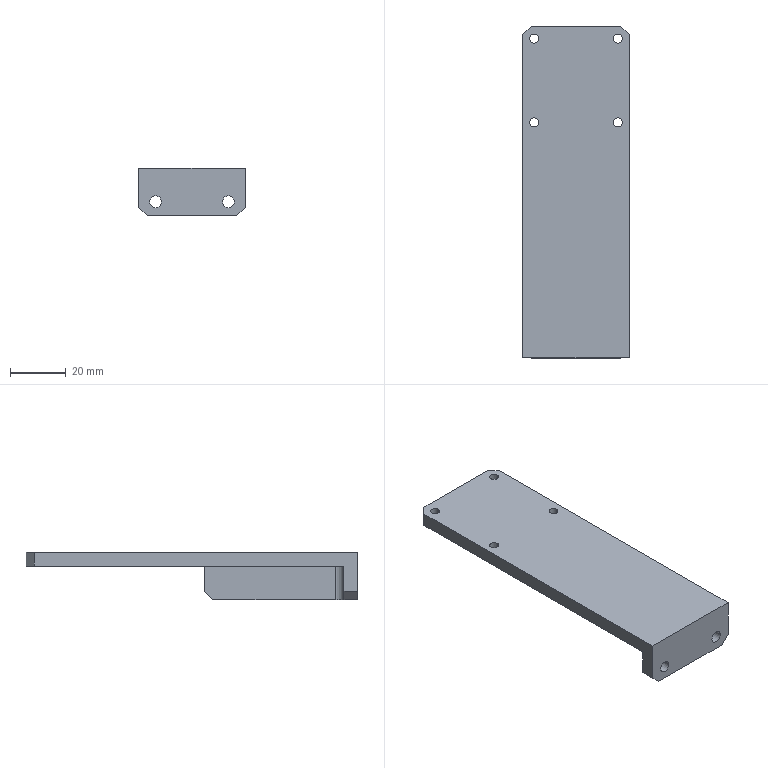NC program | NX | posted with a generic post | part box 38.1 x 118.8 x 17 mm
Lines 1 to 1973 of 2704, first 1714 of 1959 lines:
N10 G17 G21 G94 G90
(FLOOR_WALL_COPY_COPY , TOOL : D80)
N12 T19 M6
N14 G54
N16 G17 G0 G90 X-104.4 Y0. S6500 M3
N18 G43 Z30. H19
N20 Z5.
N22 G94 G1 Z2. F1500.
N24 X-99.4
N26 X99.4
N28 X104.4
N30 Z5.
N32 G0 Z30.
N34 X-104.4
N36 Z4.
N38 G1 Z1.
N40 X-99.4
N42 X99.4
N44 X104.4
N46 Z4.
N48 G0 Z30.
N50 X-104.4
N52 Z3.
N54 G1 Z0.
N56 X-99.4
N58 X99.4
N60 X104.4
N62 Z3.
N64 G0 Z30.
N66 M5
(FLOOR_WALL , TOOL : D10)
N68 T15 M6
N70 G54
N72 G17 G0 G90 X63.9 Y-22.864 S9500 M3
N74 G43 Z30. H15
N76 Z-8.9
N78 G94 G1 Z-10.9 F1000.
N80 Y-22.788 Z-11.283
N82 Y-22.571 Z-11.607
N84 Y-22.246 Z-11.824
N86 Y-21.864 Z-11.9
N88 Y-18.621
N90 Y18.518 F3000.
N92 X63.909 Y18.625
N94 X63.827 Y18.694
N96 X63.572 Y18.949
N98 G3 X63.402 Y18.878 R0.1
N100 G1 Y-19.016
N102 X63.41 Y-19.123
N104 X63.328 Y-19.193
N106 X63.074 Y-19.447
N108 G2 X62.903 Y-19.377 R0.1
N110 G1 Y19.515
N112 X62.912 Y19.622
N114 X62.83 Y19.691
N116 X62.575 Y19.946
N118 G3 X62.405 Y19.875 R0.1
N120 G1 Y-20.013
N122 X62.413 Y-20.12
N124 X62.332 Y-20.189
N126 X62.077 Y-20.444
N128 G2 X61.906 Y-20.374 R0.1
N130 G1 Y20.512
N132 X61.915 Y20.619
N134 X61.833 Y20.688
N136 X61.578 Y20.943
N138 G3 X61.408 Y20.872 R0.1
N140 G1 Y-21.01
N142 X61.416 Y-21.117
N144 X61.335 Y-21.186
N146 X61.08 Y-21.441
N148 G2 X60.909 Y-21.371 R0.1
N150 G1 Y21.509
N152 X60.918 Y21.615
N154 X60.836 Y21.685
N156 X60.581 Y21.94
N158 G3 X60.411 Y21.869 R0.1
N160 G1 Y-22.007
N162 X60.419 Y-22.114
N164 X60.338 Y-22.183
N166 X60.083 Y-22.438
N168 G2 X59.912 Y-22.367 R0.1
N170 G1 Y22.505
N172 X59.921 Y22.612
N174 X59.839 Y22.682
N176 X59.584 Y22.937
N178 G3 X59.414 Y22.866 R0.1
N180 G1 Y-23.004
N182 X59.423 Y-23.111
N184 X59.341 Y-23.18
N186 X59.086 Y-23.435
N188 G2 X58.915 Y-23.364 R0.1
N190 G1 Y23.502
N192 X58.924 Y23.609
N194 X58.842 Y23.679
N196 X58.588 Y23.934
N198 G3 X58.417 Y23.863 R0.1
N200 G1 Y-23.826
N202 G2 X58.193 Y-24.05 R0.224
N204 G1 X58.168
N206 G2 X57.918 Y-23.8 R0.25
N208 G1 Y23.826
N210 G3 X57.694 Y24.05 R0.224
N212 G1 X57.67
N214 G3 X57.42 Y23.8 R0.25
N216 G1 Y-23.826
N218 G2 X57.196 Y-24.05 R0.224
N220 G1 X57.172
N222 G2 X56.922 Y-23.8 R0.25
N224 G1 Y23.826
N226 G3 X56.697 Y24.05 R0.224
N228 G1 X56.673
N230 G3 X56.423 Y23.8 R0.25
N232 G1 Y-23.826
N234 G2 X56.199 Y-24.05 R0.224
N236 G1 X56.175
N238 G2 X55.925 Y-23.8 R0.25
N240 G1 Y23.826
N242 G3 X55.7 Y24.05 R0.224
N244 G1 X55.676
N246 G3 X55.426 Y23.8 R0.25
N248 G1 Y-23.826
N250 G2 X55.202 Y-24.05 R0.224
N252 G1 X55.178
N254 G2 X54.928 Y-23.8 R0.25
N256 G1 Y23.826
N258 G3 X54.703 Y24.05 R0.224
N260 G1 X54.679
N262 G3 X54.429 Y23.8 R0.25
N264 G1 Y-23.826
N266 G2 X54.205 Y-24.05 R0.224
N268 G1 X54.181
N270 G2 X53.931 Y-23.8 R0.25
N272 G1 Y23.826
N274 G3 X53.707 Y24.05 R0.224
N276 G1 X53.682
N278 G3 X53.432 Y23.8 R0.25
N280 G1 Y-23.826
N282 G2 X53.208 Y-24.05 R0.224
N284 G1 X53.184
N286 G2 X52.934 Y-23.8 R0.25
N288 G1 Y23.826
N290 G3 X52.71 Y24.05 R0.224
N292 G1 X52.685
N294 G3 X52.435 Y23.8 R0.25
N296 G1 Y-23.826
N298 G2 X52.211 Y-24.05 R0.224
N300 G1 X52.187
N302 G2 X51.937 Y-23.8 R0.25
N304 G1 Y23.826
N306 G3 X51.713 Y24.05 R0.224
N308 G1 X51.689
N310 G3 X51.439 Y23.8 R0.25
N312 G1 Y-23.826
N314 G2 X51.214 Y-24.05 R0.224
N316 G1 X51.19
N318 G2 X50.94 Y-23.8 R0.25
N320 G1 Y23.826
N322 G3 X50.716 Y24.05 R0.224
N324 G1 X50.692
N326 G3 X50.442 Y23.8 R0.25
N328 G1 Y-23.826
N330 G2 X50.217 Y-24.05 R0.224
N332 G1 X50.193
N334 G2 X49.943 Y-23.8 R0.25
N336 G1 Y23.826
N338 G3 X49.719 Y24.05 R0.224
N340 G1 X49.695
N342 G3 X49.445 Y23.8 R0.25
N344 G1 Y-23.826
N346 G2 X49.22 Y-24.05 R0.224
N348 G1 X49.196
N350 G2 X48.946 Y-23.8 R0.25
N352 G1 Y23.826
N354 G3 X48.722 Y24.05 R0.224
N356 G1 X48.698
N358 G3 X48.448 Y23.8 R0.25
N360 G1 Y-23.826
N362 G2 X48.223 Y-24.05 R0.224
N364 G1 X48.199
N366 G2 X47.949 Y-23.8 R0.25
N368 G1 Y23.826
N370 G3 X47.725 Y24.05 R0.224
N372 G1 X47.701
N374 G3 X47.451 Y23.8 R0.25
N376 G1 Y-23.826
N378 G2 X47.227 Y-24.05 R0.224
N380 G1 X47.202
N382 G2 X46.952 Y-23.8 R0.25
N384 G1 Y23.826
N386 G3 X46.728 Y24.05 R0.224
N388 G1 X46.704
N390 G3 X46.454 Y23.8 R0.25
N392 G1 Y-23.826
N394 G2 X46.23 Y-24.05 R0.224
N396 G1 X46.205
N398 G2 X45.955 Y-23.8 R0.25
N400 G1 Y23.826
N402 G3 X45.731 Y24.05 R0.224
N404 G1 X45.707
N406 G3 X45.457 Y23.8 R0.25
N408 G1 Y-23.826
N410 G2 X45.233 Y-24.05 R0.224
N412 G1 X45.209
N414 G2 X44.959 Y-23.8 R0.25
N416 G1 Y23.826
N418 G3 X44.734 Y24.05 R0.224
N420 G1 X44.71
N422 G3 X44.46 Y23.8 R0.25
N424 G1 Y-23.826
N426 G2 X44.236 Y-24.05 R0.224
N428 G1 X44.212
N430 G2 X43.962 Y-23.8 R0.25
N432 G1 Y23.826
N434 G3 X43.737 Y24.05 R0.224
N436 G1 X43.713
N438 G3 X43.463 Y23.8 R0.25
N440 G1 Y-23.826
N442 G2 X43.239 Y-24.05 R0.224
N444 G1 X43.215
N446 G2 X42.965 Y-23.8 R0.25
N448 G1 Y23.826
N450 G3 X42.74 Y24.05 R0.224
N452 G1 X42.716
N454 G3 X42.466 Y23.8 R0.25
N456 G1 Y-23.826
N458 G2 X42.242 Y-24.05 R0.224
N460 G1 X42.218
N462 G2 X41.968 Y-23.8 R0.25
N464 G1 Y23.826
N466 G3 X41.744 Y24.05 R0.224
N468 G1 X41.719
N470 G3 X41.469 Y23.8 R0.25
N472 G1 Y-23.826
N474 G2 X41.245 Y-24.05 R0.224
N476 G1 X41.221
N478 G2 X40.971 Y-23.8 R0.25
N480 G1 Y23.826
N482 G3 X40.747 Y24.05 R0.224
N484 G1 X40.722
N486 G3 X40.472 Y23.8 R0.25
N488 G1 Y-23.826
N490 G2 X40.248 Y-24.05 R0.224
N492 G1 X40.224
N494 G2 X39.974 Y-23.8 R0.25
N496 G1 Y23.826
N498 G3 X39.75 Y24.05 R0.224
N500 G1 X39.726
N502 G3 X39.476 Y23.8 R0.25
N504 G1 Y-23.826
N506 G2 X39.251 Y-24.05 R0.224
N508 G1 X39.227
N510 G2 X38.977 Y-23.8 R0.25
N512 G1 Y23.826
N514 G3 X38.753 Y24.05 R0.224
N516 G1 X38.729
N518 G3 X38.479 Y23.8 R0.25
N520 G1 Y-23.826
N522 G2 X38.254 Y-24.05 R0.224
N524 G1 X38.23
N526 G2 X37.98 Y-23.8 R0.25
N528 G1 Y23.826
N530 G3 X37.756 Y24.05 R0.224
N532 G1 X37.732
N534 G3 X37.482 Y23.8 R0.25
N536 G1 Y-23.826
N538 G2 X37.257 Y-24.05 R0.224
N540 G1 X37.233
N542 G2 X36.983 Y-23.8 R0.25
N544 G1 Y23.826
N546 G3 X36.759 Y24.05 R0.224
N548 G1 X36.735
N550 G3 X36.485 Y23.8 R0.25
N552 G1 Y-23.826
N554 G2 X36.26 Y-24.05 R0.224
N556 G1 X36.236
N558 G2 X35.986 Y-23.8 R0.25
N560 G1 Y23.826
N562 G3 X35.762 Y24.05 R0.224
N564 G1 X35.738
N566 G3 X35.488 Y23.8 R0.25
N568 G1 Y-23.826
N570 G2 X35.264 Y-24.05 R0.224
N572 G1 X35.239
N574 G2 X34.989 Y-23.8 R0.25
N576 G1 Y23.826
N578 G3 X34.765 Y24.05 R0.224
N580 G1 X34.741
N582 G3 X34.491 Y23.8 R0.25
N584 G1 Y-23.826
N586 G2 X34.267 Y-24.05 R0.224
N588 G1 X34.243
N590 G2 X33.993 Y-23.8 R0.25
N592 G1 Y23.826
N594 G3 X33.768 Y24.05 R0.224
N596 G1 X33.744
N598 G3 X33.494 Y23.8 R0.25
N600 G1 Y-23.826
N602 G2 X33.27 Y-24.05 R0.224
N604 G1 X33.246
N606 G2 X32.996 Y-23.8 R0.25
N608 G1 Y23.826
N610 G3 X32.771 Y24.05 R0.224
N612 G1 X32.747
N614 G3 X32.497 Y23.8 R0.25
N616 G1 Y-23.826
N618 G2 X32.273 Y-24.05 R0.224
N620 G1 X32.249
N622 G2 X31.999 Y-23.8 R0.25
N624 G1 Y23.826
N626 G3 X31.774 Y24.05 R0.224
N628 G1 X31.75
N630 G3 X31.5 Y23.8 R0.25
N632 G1 Y-23.826
N634 G2 X31.276 Y-24.05 R0.224
N636 G1 X31.252
N638 G2 X31.002 Y-23.8 R0.25
N640 G1 Y23.826
N642 G3 X30.777 Y24.05 R0.224
N644 G1 X30.753
N646 G3 X30.503 Y23.8 R0.25
N648 G1 Y-23.826
N650 G2 X30.279 Y-24.05 R0.224
N652 G1 X30.255
N654 G2 X30.005 Y-23.8 R0.25
N656 G1 Y23.826
N658 G3 X29.781 Y24.05 R0.224
N660 G1 X29.756
N662 G3 X29.506 Y23.8 R0.25
N664 G1 Y-23.826
N666 G2 X29.282 Y-24.05 R0.224
N668 G1 X29.258
N670 G2 X29.008 Y-23.8 R0.25
N672 G1 Y23.826
N674 G3 X28.784 Y24.05 R0.224
N676 G1 X28.759
N678 G3 X28.509 Y23.8 R0.25
N680 G1 Y-23.826
N682 G2 X28.285 Y-24.05 R0.224
N684 G1 X28.261
N686 G2 X28.011 Y-23.8 R0.25
N688 G1 Y23.826
N690 G3 X27.787 Y24.05 R0.224
N692 G1 X27.763
N694 G3 X27.513 Y23.8 R0.25
N696 G1 Y-23.826
N698 G2 X27.288 Y-24.05 R0.224
N700 G1 X27.264
N702 G2 X27.014 Y-23.8 R0.25
N704 G1 Y23.826
N706 G3 X26.79 Y24.05 R0.224
N708 G1 X26.766
N710 G3 X26.516 Y23.8 R0.25
N712 G1 Y-23.826
N714 G2 X26.291 Y-24.05 R0.224
N716 G1 X26.267
N718 G2 X26.017 Y-23.8 R0.25
N720 G1 Y23.826
N722 G3 X25.793 Y24.05 R0.224
N724 G1 X25.769
N726 G3 X25.519 Y23.8 R0.25
N728 G1 Y-23.826
N730 G2 X25.294 Y-24.05 R0.224
N732 G1 X25.27
N734 G2 X25.02 Y-23.8 R0.25
N736 G1 Y23.826
N738 G3 X24.796 Y24.05 R0.224
N740 G1 X24.772
N742 G3 X24.522 Y23.8 R0.25
N744 G1 Y-23.826
N746 G2 X24.297 Y-24.05 R0.224
N748 G1 X24.273
N750 G2 X24.023 Y-23.8 R0.25
N752 G1 Y23.826
N754 G3 X23.799 Y24.05 R0.224
N756 G1 X23.775
N758 G3 X23.525 Y23.8 R0.25
N760 G1 Y-23.826
N762 G2 X23.301 Y-24.05 R0.224
N764 G1 X23.276
N766 G2 X23.026 Y-23.8 R0.25
N768 G1 Y23.826
N770 G3 X22.802 Y24.05 R0.224
N772 G1 X22.778
N774 G3 X22.528 Y23.8 R0.25
N776 G1 Y-23.826
N778 G2 X22.304 Y-24.05 R0.224
N780 G1 X22.28
N782 G2 X22.03 Y-23.8 R0.25
N784 G1 Y23.826
N786 G3 X21.805 Y24.05 R0.224
N788 G1 X21.781
N790 G3 X21.531 Y23.8 R0.25
N792 G1 Y-23.826
N794 G2 X21.307 Y-24.05 R0.224
N796 G1 X21.283
N798 G2 X21.033 Y-23.8 R0.25
N800 G1 Y23.826
N802 G3 X20.808 Y24.05 R0.224
N804 G1 X20.784
N806 G3 X20.534 Y23.8 R0.25
N808 G1 Y-23.826
N810 G2 X20.31 Y-24.05 R0.224
N812 G1 X20.286
N814 G2 X20.036 Y-23.8 R0.25
N816 G1 Y23.826
N818 G3 X19.811 Y24.05 R0.224
N820 G1 X19.787
N822 G3 X19.537 Y23.8 R0.25
N824 G1 Y-23.826
N826 G2 X19.313 Y-24.05 R0.224
N828 G1 X19.289
N830 G2 X19.039 Y-23.8 R0.25
N832 G1 Y23.826
N834 G3 X18.814 Y24.05 R0.224
N836 G1 X18.79
N838 G3 X18.54 Y23.8 R0.25
N840 G1 Y-23.826
N842 G2 X18.316 Y-24.05 R0.224
N844 G1 X18.292
N846 G2 X18.042 Y-23.8 R0.25
N848 G1 Y23.826
N850 G3 X17.818 Y24.05 R0.224
N852 G1 X17.793
N854 G3 X17.543 Y23.8 R0.25
N856 G1 Y-23.826
N858 G2 X17.319 Y-24.05 R0.224
N860 G1 X17.295
N862 G2 X17.045 Y-23.8 R0.25
N864 G1 Y23.826
N866 G3 X16.821 Y24.05 R0.224
N868 G1 X16.796
N870 G3 X16.546 Y23.8 R0.25
N872 G1 Y-23.826
N874 G2 X16.322 Y-24.05 R0.224
N876 G1 X16.298
N878 G2 X16.048 Y-23.8 R0.25
N880 G1 Y23.826
N882 G3 X15.824 Y24.05 R0.224
N884 G1 X15.8
N886 G3 X15.55 Y23.8 R0.25
N888 G1 Y-23.826
N890 G2 X15.325 Y-24.05 R0.224
N892 G1 X15.301
N894 G2 X15.051 Y-23.8 R0.25
N896 G1 Y23.826
N898 G3 X14.827 Y24.05 R0.224
N900 G1 X14.803
N902 G3 X14.553 Y23.8 R0.25
N904 G1 Y-23.826
N906 G2 X14.328 Y-24.05 R0.224
N908 G1 X14.304
N910 G2 X14.054 Y-23.8 R0.25
N912 G1 Y23.826
N914 G3 X13.83 Y24.05 R0.224
N916 G1 X13.806
N918 G3 X13.556 Y23.8 R0.25
N920 G1 Y-23.826
N922 G2 X13.331 Y-24.05 R0.224
N924 G1 X13.307
N926 G2 X13.057 Y-23.8 R0.25
N928 G1 Y23.826
N930 G3 X12.833 Y24.05 R0.224
N932 G1 X12.809
N934 G3 X12.559 Y23.8 R0.25
N936 G1 Y-23.826
N938 G2 X12.335 Y-24.05 R0.224
N940 G1 X12.31
N942 G2 X12.06 Y-23.8 R0.25
N944 G1 Y23.826
N946 G3 X11.836 Y24.05 R0.224
N948 G1 X11.812
N950 G3 X11.562 Y23.8 R0.25
N952 G1 Y-23.826
N954 G2 X11.338 Y-24.05 R0.224
N956 G1 X11.313
N958 G2 X11.063 Y-23.8 R0.25
N960 G1 Y23.826
N962 G3 X10.839 Y24.05 R0.224
N964 G1 X10.815
N966 G3 X10.565 Y23.8 R0.25
N968 G1 Y-23.826
N970 G2 X10.341 Y-24.05 R0.224
N972 G1 X10.317
N974 G2 X10.067 Y-23.8 R0.25
N976 G1 Y23.826
N978 G3 X9.842 Y24.05 R0.224
N980 G1 X9.818
N982 G3 X9.568 Y23.8 R0.25
N984 G1 Y-23.826
N986 G2 X9.344 Y-24.05 R0.224
N988 G1 X9.32
N990 G2 X9.07 Y-23.8 R0.25
N992 G1 Y23.826
N994 G3 X8.845 Y24.05 R0.224
N996 G1 X8.821
N998 G3 X8.571 Y23.8 R0.25
N1000 G1 Y-23.826
N1002 G2 X8.347 Y-24.05 R0.224
N1004 G1 X8.323
N1006 G2 X8.073 Y-23.8 R0.25
N1008 G1 Y23.826
N1010 G3 X7.848 Y24.05 R0.224
N1012 G1 X7.824
N1014 G3 X7.574 Y23.8 R0.25
N1016 G1 Y-23.826
N1018 G2 X7.35 Y-24.05 R0.224
N1020 G1 X7.326
N1022 G2 X7.076 Y-23.8 R0.25
N1024 G1 Y23.826
N1026 G3 X6.851 Y24.05 R0.224
N1028 G1 X6.827
N1030 G3 X6.577 Y23.8 R0.25
N1032 G1 Y-23.826
N1034 G2 X6.353 Y-24.05 R0.224
N1036 G1 X6.329
N1038 G2 X6.079 Y-23.8 R0.25
N1040 G1 Y23.826
N1042 G3 X5.855 Y24.05 R0.224
N1044 G1 X5.83
N1046 G3 X5.58 Y23.8 R0.25
N1048 G1 Y-23.826
N1050 G2 X5.356 Y-24.05 R0.224
N1052 G1 X5.332
N1054 G2 X5.082 Y-23.8 R0.25
N1056 G1 Y23.826
N1058 G3 X4.858 Y24.05 R0.224
N1060 G1 X4.833
N1062 G3 X4.583 Y23.8 R0.25
N1064 G1 Y-23.826
N1066 G2 X4.359 Y-24.05 R0.224
N1068 G1 X4.335
N1070 G2 X4.085 Y-23.8 R0.25
N1072 G1 Y23.826
N1074 G3 X3.861 Y24.05 R0.224
N1076 G1 X3.837
N1078 G3 X3.587 Y23.8 R0.25
N1080 G1 Y-23.826
N1082 G2 X3.362 Y-24.05 R0.224
N1084 G1 X3.338
N1086 G2 X3.088 Y-23.8 R0.25
N1088 G1 Y23.826
N1090 G3 X2.864 Y24.05 R0.224
N1092 G1 X2.84
N1094 G3 X2.59 Y23.8 R0.25
N1096 G1 Y-23.826
N1098 G2 X2.365 Y-24.05 R0.224
N1100 G1 X2.341
N1102 G2 X2.091 Y-23.8 R0.25
N1104 G1 Y23.826
N1106 G3 X1.867 Y24.05 R0.224
N1108 G1 X1.843
N1110 G3 X1.593 Y23.8 R0.25
N1112 G1 Y-23.826
N1114 G2 X1.368 Y-24.05 R0.224
N1116 G1 X1.344
N1118 G2 X1.094 Y-23.8 R0.25
N1120 G1 Y23.826
N1122 G3 X0.87 Y24.05 R0.224
N1124 G1 X0.846
N1126 G3 X0.596 Y23.8 R0.25
N1128 G1 Y9.374
N1130 G2 X0.372 Y9.15 R0.224
N1132 G1 X0.347
N1134 G2 X0.097 Y9.4 R0.25
N1136 G1 Y23.826
N1138 G3 X-0.127 Y24.05 R0.224
N1140 G1 X-0.151
N1142 G3 X-0.401 Y23.8 R0.25
N1144 G1 Y9.399
N1146 G2 X-0.65 Y9.15 R0.249
N1148 G1 X-0.675
N1150 G2 X-0.9 Y9.374 R0.224
N1152 G1 Y23.826
N1154 G3 X-1.124 Y24.05 R0.224
N1156 G1 X-1.148
N1158 G3 X-1.398 Y23.8 R0.25
N1160 G1 Y9.399
N1162 G2 X-1.647 Y9.15 R0.249
N1164 G1 X-1.672
N1166 G2 X-1.896 Y9.374 R0.224
N1168 G1 Y23.826
N1170 G3 X-2.121 Y24.05 R0.224
N1172 G1 X-2.145
N1174 G3 X-2.395 Y23.8 R0.25
N1176 G1 Y9.399
N1178 G2 X-2.644 Y9.15 R0.249
N1180 G1 X-2.669
N1182 G2 X-2.893 Y9.374 R0.224
N1184 G1 Y23.826
N1186 G3 X-3.118 Y24.05 R0.224
N1188 G1 X-3.142
N1190 G3 X-3.392 Y23.8 R0.25
N1192 G1 Y9.374
N1194 G2 X-3.616 Y9.15 R0.224
N1196 G1 X-3.64
N1198 G2 X-3.89 Y9.4 R0.25
N1200 G1 Y23.826
N1202 G3 X-4.115 Y24.05 R0.224
N1204 G1 X-4.139
N1206 G3 X-4.389 Y23.8 R0.25
N1208 G1 Y9.374
N1210 G2 X-4.613 Y9.15 R0.224
N1212 G1 X-4.637
N1214 G2 X-4.887 Y9.4 R0.25
N1216 G1 Y23.826
N1218 G3 X-5.112 Y24.05 R0.224
N1220 G1 X-5.136
N1222 G3 X-5.386 Y23.8 R0.25
N1224 G1 Y9.374
N1226 G2 X-5.61 Y9.15 R0.224
N1228 G1 X-5.634
N1230 G2 X-5.884 Y9.4 R0.25
N1232 G1 Y23.826
N1234 G3 X-6.108 Y24.05 R0.224
N1236 G1 X-6.133
N1238 G3 X-6.383 Y23.8 R0.25
N1240 G1 Y9.374
N1242 G2 X-6.607 Y9.15 R0.224
N1244 G1 X-6.631
N1246 G2 X-6.881 Y9.4 R0.25
N1248 G1 Y23.826
N1250 G3 X-7.105 Y24.05 R0.224
N1252 G1 X-7.13
N1254 G3 X-7.38 Y23.8 R0.25
N1256 G1 Y9.374
N1258 G2 X-7.604 Y9.15 R0.224
N1260 G1 X-7.628
N1262 G2 X-7.878 Y9.4 R0.25
N1264 G1 Y23.826
N1266 G3 X-8.102 Y24.05 R0.224
N1268 G1 X-8.126
N1270 G3 X-8.376 Y23.8 R0.25
N1272 G1 Y9.374
N1274 G2 X-8.601 Y9.15 R0.224
N1276 G1 X-8.625
N1278 G2 X-8.875 Y9.4 R0.25
N1280 G1 Y23.826
N1282 G3 X-9.099 Y24.05 R0.224
N1284 G1 X-9.123
N1286 G3 X-9.373 Y23.8 R0.25
N1288 G1 Y9.374
N1290 G2 X-9.598 Y9.15 R0.224
N1292 G1 X-9.622
N1294 G2 X-9.872 Y9.4 R0.25
N1296 G1 Y23.826
N1298 G3 X-10.096 Y24.05 R0.224
N1300 G1 X-10.12
N1302 G3 X-10.37 Y23.8 R0.25
N1304 G1 Y9.374
N1306 G2 X-10.595 Y9.15 R0.224
N1308 G1 X-10.619
N1310 G2 X-10.869 Y9.4 R0.25
N1312 G1 Y23.826
N1314 G3 X-11.093 Y24.05 R0.224
N1316 G1 X-11.117
N1318 G3 X-11.367 Y23.8 R0.25
N1320 G1 Y9.374
N1322 G2 X-11.591 Y9.15 R0.224
N1324 G1 X-11.616
N1326 G2 X-11.866 Y9.4 R0.25
N1328 G1 Y23.826
N1330 G3 X-12.09 Y24.05 R0.224
N1332 G1 X-12.114
N1334 G3 X-12.364 Y23.8 R0.25
N1336 G1 Y9.374
N1338 G2 X-12.588 Y9.15 R0.224
N1340 G1 X-12.613
N1342 G2 X-12.863 Y9.4 R0.25
N1344 G1 Y23.826
N1346 G3 X-13.087 Y24.05 R0.224
N1348 G1 X-13.111
N1350 G3 X-13.361 Y23.8 R0.25
N1352 G1 Y9.399
N1354 G2 X-13.61 Y9.15 R0.249
N1356 G1 X-13.635
N1358 G2 X-13.859 Y9.374 R0.224
N1360 G1 Y23.826
N1362 G3 X-14.084 Y24.05 R0.224
N1364 G1 X-14.108
N1366 G3 X-14.358 Y23.8 R0.25
N1368 G1 Y9.374
N1370 G2 X-14.582 Y9.15 R0.224
N1372 G1 X-14.606
N1374 G2 X-14.856 Y9.4 R0.25
N1376 G1 Y23.826
N1378 G3 X-15.081 Y24.05 R0.224
N1380 G1 X-15.105
N1382 G3 X-15.355 Y23.8 R0.25
N1384 G1 Y9.374
N1386 G2 X-15.579 Y9.15 R0.224
N1388 G1 X-15.603
N1390 G2 X-15.853 Y9.4 R0.25
N1392 G1 Y23.826
N1394 G3 X-16.078 Y24.05 R0.224
N1396 G1 X-16.102
N1398 G3 X-16.352 Y23.8 R0.25
N1400 G1 Y9.374
N1402 G2 X-16.576 Y9.15 R0.224
N1404 G1 X-16.6
N1406 G2 X-16.85 Y9.4 R0.25
N1408 G1 Y23.826
N1410 G3 X-17.075 Y24.05 R0.224
N1412 G1 X-17.099
N1414 G3 X-17.349 Y23.8 R0.25
N1416 G1 Y9.374
N1418 G2 X-17.573 Y9.15 R0.224
N1420 G1 X-17.597
N1422 G2 X-17.847 Y9.4 R0.25
N1424 G1 Y23.826
N1426 G3 X-18.071 Y24.05 R0.224
N1428 G1 X-18.096
N1430 G3 X-18.346 Y23.8 R0.25
N1432 G1 Y9.374
N1434 G2 X-18.57 Y9.15 R0.224
N1436 G1 X-18.594
N1438 G2 X-18.844 Y9.4 R0.25
N1440 G1 Y23.826
N1442 G3 X-19.068 Y24.05 R0.224
N1444 G1 X-19.093
N1446 G3 X-19.343 Y23.8 R0.25
N1448 G1 Y9.374
N1450 G2 X-19.567 Y9.15 R0.224
N1452 G1 X-19.591
N1454 G2 X-19.841 Y9.4 R0.25
N1456 G1 Y23.826
N1458 G3 X-20.065 Y24.05 R0.224
N1460 G1 X-20.089
N1462 G3 X-20.339 Y23.8 R0.25
N1464 G1 Y9.374
N1466 G2 X-20.564 Y9.15 R0.224
N1468 G1 X-20.588
N1470 G2 X-20.838 Y9.4 R0.25
N1472 G1 Y23.826
N1474 G3 X-21.062 Y24.05 R0.224
N1476 G1 X-21.086
N1478 G3 X-21.336 Y23.8 R0.25
N1480 G1 Y9.374
N1482 G2 X-21.561 Y9.15 R0.224
N1484 G1 X-21.585
N1486 G2 X-21.835 Y9.4 R0.25
N1488 G1 Y23.826
N1490 G3 X-22.059 Y24.05 R0.224
N1492 G1 X-22.083
N1494 G3 X-22.333 Y23.8 R0.25
N1496 G1 Y9.374
N1498 G2 X-22.558 Y9.15 R0.224
N1500 G1 X-22.582
N1502 G2 X-22.832 Y9.4 R0.25
N1504 G1 Y23.826
N1506 G3 X-23.056 Y24.05 R0.224
N1508 G1 X-23.08
N1510 G3 X-23.33 Y23.8 R0.25
N1512 G1 Y9.399
N1514 G2 X-23.579 Y9.15 R0.249
N1516 G1 X-23.604
N1518 G2 X-23.829 Y9.374 R0.224
N1520 G1 Y23.826
N1522 G3 X-24.053 Y24.05 R0.224
N1524 G1 X-24.077
N1526 G3 X-24.327 Y23.8 R0.25
N1528 G1 Y9.374
N1530 G2 X-24.551 Y9.15 R0.224
N1532 G1 X-24.576
N1534 G2 X-24.826 Y9.4 R0.25
N1536 G1 Y23.826
N1538 G3 X-25.05 Y24.05 R0.224
N1540 G1 X-25.074
N1542 G3 X-25.324 Y23.8 R0.25
N1544 G1 Y9.374
N1546 G2 X-25.548 Y9.15 R0.224
N1548 G1 X-25.572
N1550 G2 X-25.822 Y9.4 R0.25
N1552 G1 Y23.826
N1554 G3 X-26.047 Y24.05 R0.224
N1556 G1 X-26.071
N1558 G3 X-26.321 Y23.8 R0.25
N1560 G1 Y9.374
N1562 G2 X-26.545 Y9.15 R0.224
N1564 G1 X-26.569
N1566 G2 X-26.819 Y9.4 R0.25
N1568 G1 Y23.826
N1570 G3 X-27.044 Y24.05 R0.224
N1572 G1 X-27.068
N1574 G3 X-27.318 Y23.8 R0.25
N1576 G1 Y9.374
N1578 G2 X-27.542 Y9.15 R0.224
N1580 G1 X-27.566
N1582 G2 X-27.816 Y9.4 R0.25
N1584 G1 Y23.826
N1586 G3 X-28.041 Y24.05 R0.224
N1588 G1 X-28.065
N1590 G3 X-28.315 Y23.8 R0.25
N1592 G1 Y9.374
N1594 G2 X-28.539 Y9.15 R0.224
N1596 G1 X-28.563
N1598 G2 X-28.813 Y9.4 R0.25
N1600 G1 Y23.826
N1602 G3 X-29.038 Y24.05 R0.224
N1604 G1 X-29.062
N1606 G3 X-29.312 Y23.8 R0.25
N1608 G1 Y9.399
N1610 G2 X-29.561 Y9.15 R0.249
N1612 G1 X-29.586
N1614 G2 X-29.81 Y9.374 R0.224
N1616 G1 Y23.826
N1618 G3 X-30.034 Y24.05 R0.224
N1620 G1 X-30.059
N1622 G3 X-30.309 Y23.8 R0.25
N1624 G1 Y9.374
N1626 G2 X-30.533 Y9.15 R0.224
N1628 G1 X-30.557
N1630 G2 X-30.807 Y9.4 R0.25
N1632 G1 Y23.826
N1634 G3 X-31.031 Y24.05 R0.224
N1636 G1 X-31.055
N1638 G3 X-31.305 Y23.8 R0.25
N1640 G1 Y9.374
N1642 G2 X-31.53 Y9.15 R0.224
N1644 G1 X-31.554
N1646 G2 X-31.804 Y9.4 R0.25
N1648 G1 Y23.826
N1650 G3 X-32.028 Y24.05 R0.224
N1652 G1 X-32.052
N1654 G3 X-32.302 Y23.8 R0.25
N1656 G1 Y9.374
N1658 G2 X-32.527 Y9.15 R0.224
N1660 G1 X-32.551
N1662 G2 X-32.801 Y9.4 R0.25
N1664 G1 Y23.826
N1666 G3 X-33.025 Y24.05 R0.224
N1668 G1 X-33.049
N1670 G3 X-33.299 Y23.8 R0.25
N1672 G1 Y9.374
N1674 G2 X-33.524 Y9.15 R0.224
N1676 G1 X-33.548
N1678 G2 X-33.798 Y9.4 R0.25
N1680 G1 Y23.826
N1682 G3 X-34.022 Y24.05 R0.224
N1684 G1 X-34.046
N1686 G3 X-34.296 Y23.8 R0.25
N1688 G1 Y9.374
N1690 G2 X-34.521 Y9.15 R0.224
N1692 G1 X-34.545
N1694 G2 X-34.795 Y9.4 R0.25
N1696 G1 Y23.826
N1698 G3 X-35.019 Y24.05 R0.224
N1700 G1 X-35.043
N1702 G3 X-35.293 Y23.8 R0.25
N1704 G1 Y9.374
N1706 G2 X-35.517 Y9.15 R0.224
N1708 G1 X-35.542
N1710 G2 X-35.792 Y9.4 R0.25
N1712 G1 Y23.826
N1714 G3 X-36.016 Y24.05 R0.224
N1716 G1 X-36.04
N1718 G3 X-36.29 Y23.8 R0.25
N1720 G1 Y9.374
N1722 G2 X-36.514 Y9.15 R0.224
N1724 G1 X-36.539
N1726 G2 X-36.789 Y9.4 R0.25
N1728 G1 Y23.826
N1730 G3 X-37.013 Y24.05 R0.224
N1732 G1 X-37.037
N1734 G3 X-37.287 Y23.8 R0.25
N1736 G1 Y9.374
N1738 G2 X-37.511 Y9.15 R0.224
N1740 G1 X-37.535
N1742 G2 X-37.785 Y9.4 R0.25
N1744 G1 Y23.826
N1746 G3 X-38.01 Y24.05 R0.224
N1748 G1 X-38.034
N1750 G3 X-38.284 Y23.8 R0.25
N1752 G1 Y9.374
N1754 G2 X-38.508 Y9.15 R0.224
N1756 G1 X-38.532
N1758 G2 X-38.782 Y9.4 R0.25
N1760 G1 Y23.826
N1762 G3 X-39.007 Y24.05 R0.224
N1764 G1 X-39.031
N1766 G3 X-39.281 Y23.8 R0.25
N1768 G1 Y9.374
N1770 G2 X-39.505 Y9.15 R0.224
N1772 G1 X-39.529
N1774 G2 X-39.779 Y9.4 R0.25
N1776 G1 Y23.826
N1778 G3 X-40.004 Y24.05 R0.224
N1780 G1 X-40.028
N1782 G3 X-40.278 Y23.8 R0.25
N1784 G1 Y9.374
N1786 G2 X-40.502 Y9.15 R0.224
N1788 G1 X-40.526
N1790 G2 X-40.776 Y9.4 R0.25
N1792 G1 Y23.826
N1794 G3 X-41.001 Y24.05 R0.224
N1796 G1 X-41.025
N1798 G3 X-41.275 Y23.8 R0.25
N1800 G1 Y9.374
N1802 G2 X-41.499 Y9.15 R0.224
N1804 G1 X-41.523
N1806 G2 X-41.773 Y9.4 R0.25
N1808 G1 Y23.826
N1810 G3 X-41.997 Y24.05 R0.224
N1812 G1 X-42.022
N1814 G3 X-42.272 Y23.8 R0.25
N1816 G1 Y9.374
N1818 G2 X-42.496 Y9.15 R0.224
N1820 G1 X-42.52
N1822 G2 X-42.77 Y9.4 R0.25
N1824 G1 Y23.826
N1826 G3 X-42.994 Y24.05 R0.224
N1828 G1 X-43.018
N1830 G3 X-43.268 Y23.8 R0.25
N1832 G1 Y9.374
N1834 G2 X-43.493 Y9.15 R0.224
N1836 G1 X-43.517
N1838 G2 X-43.767 Y9.4 R0.25
N1840 G1 Y23.826
N1842 G3 X-43.991 Y24.05 R0.224
N1844 G1 X-44.015
N1846 G3 X-44.265 Y23.8 R0.25
N1848 G1 Y9.374
N1850 G2 X-44.49 Y9.15 R0.224
N1852 G1 X-44.514
N1854 G2 X-44.764 Y9.4 R0.25
N1856 G1 Y23.826
N1858 G3 X-44.988 Y24.05 R0.224
N1860 G1 X-45.012
N1862 G3 X-45.262 Y23.8 R0.25
N1864 G1 Y9.374
N1866 G2 X-45.487 Y9.15 R0.224
N1868 G1 X-45.511
N1870 G2 X-45.761 Y9.4 R0.25
N1872 G1 Y23.826
N1874 G3 X-45.985 Y24.05 R0.224
N1876 G1 X-46.009
N1878 G3 X-46.259 Y23.8 R0.25
N1880 G1 Y9.374
N1882 G2 X-46.484 Y9.15 R0.224
N1884 G1 X-46.508
N1886 G2 X-46.758 Y9.4 R0.25
N1888 G1 Y23.826
N1890 G3 X-46.982 Y24.05 R0.224
N1892 G1 X-47.006
N1894 G3 X-47.256 Y23.8 R0.25
N1896 G1 Y9.374
N1898 G2 X-47.48 Y9.15 R0.224
N1900 G1 X-47.505
N1902 G2 X-47.755 Y9.4 R0.25
N1904 G1 Y23.826
N1906 G3 X-47.979 Y24.05 R0.224
N1908 G1 X-48.003
N1910 G3 X-48.253 Y23.8 R0.25
N1912 G1 Y9.376
N1914 G2 X-48.504 Y9.183 R0.2
N1916 G1 X-48.585 Y9.208
N1918 G2 X-48.752 Y9.443 R0.25
N1920 G1 Y23.826
N1922 G3 X-48.976 Y24.05 R0.224
N1924 G1 X-49.
N1926 G3 X-49.25 Y23.8 R0.25
N1928 G1 Y10.144
N1930 Z-8.9
N1932 G0 Z29.
N1934 X-49.174 Y10.143 Z29.383
N1936 X-48.957 Y10.138 Z29.707
N1938 X-48.633 Y10.132 Z29.924
N1940 X-48.25 Y10.124 Z30.
N1942 X-0.404 Y9.17
N1944 X-0.021 Y9.162 Z29.924
N1946 X0.303 Y9.156 Z29.707
N1948 X0.52 Y9.152 Z29.383
N1950 X0.596 Y9.15 Z29.
N1952 Z-8.9
N1954 G1 Z-11.823 F1000.
N1956 X0.618 Z-11.877
N1958 X0.673 Z-11.9
N1960 X0.726 Y9.166
N1962 X0.766 Y9.126
N1964 X0.75 Y9.073
N1966 Y-9.073
N1968 X0.766 Y-9.126
N1970 X0.726 Y-9.166
N1972 X0.673 Y-9.15
N1974 X0.596
N1976 Y-23.826 F3000.
N1978 G2 X0.372 Y-24.05 R0.224
N1980 G1 X0.347
N1982 G2 X0.097 Y-23.8 R0.25
N1984 G1 Y-9.399
N1986 G3 X-0.152 Y-9.15 R0.249
N1988 G1 X-0.177
N1990 G3 X-0.401 Y-9.374 R0.224
N1992 G1 Y-23.826
N1994 G2 X-0.625 Y-24.05 R0.224
N1996 G1 X-0.65
N1998 G2 X-0.9 Y-23.8 R0.25
N2000 G1 Y-9.374
N2002 G3 X-1.124 Y-9.15 R0.224
N2004 G1 X-1.148
N2006 G3 X-1.398 Y-9.4 R0.25
N2008 G1 Y-23.826
N2010 G2 X-1.622 Y-24.05 R0.224
N2012 G1 X-1.646
N2014 G2 X-1.896 Y-23.8 R0.25
N2016 G1 Y-9.399
N2018 G3 X-2.146 Y-9.15 R0.249
N2020 G1 X-2.171
N2022 G3 X-2.395 Y-9.374 R0.224
N2024 G1 Y-23.826
N2026 G2 X-2.619 Y-24.05 R0.224
N2028 G1 X-2.643
N2030 G2 X-2.893 Y-23.8 R0.25
N2032 G1 Y-9.374
N2034 G3 X-3.118 Y-9.15 R0.224
N2036 G1 X-3.142
N2038 G3 X-3.392 Y-9.4 R0.25
N2040 G1 Y-23.826
N2042 G2 X-3.616 Y-24.05 R0.224
N2044 G1 X-3.64
N2046 G2 X-3.89 Y-23.8 R0.25
N2048 G1 Y-9.399
N2050 G3 X-4.14 Y-9.15 R0.249
N2052 G1 X-4.164
N2054 G3 X-4.389 Y-9.374 R0.224
N2056 G1 Y-23.826
N2058 G2 X-4.613 Y-24.05 R0.224
N2060 G1 X-4.637
N2062 G2 X-4.887 Y-23.8 R0.25
N2064 G1 Y-9.399
N2066 G3 X-5.136 Y-9.15 R0.249
N2068 G1 X-5.161
N2070 G3 X-5.386 Y-9.374 R0.224
N2072 G1 Y-23.826
N2074 G2 X-5.61 Y-24.05 R0.224
N2076 G1 X-5.634
N2078 G2 X-5.884 Y-23.8 R0.25
N2080 G1 Y-9.374
N2082 G3 X-6.108 Y-9.15 R0.224
N2084 G1 X-6.133
N2086 G3 X-6.383 Y-9.4 R0.25
N2088 G1 Y-23.826
N2090 G2 X-6.607 Y-24.05 R0.224
N2092 G1 X-6.631
N2094 G2 X-6.881 Y-23.8 R0.25
N2096 G1 Y-9.374
N2098 G3 X-7.105 Y-9.15 R0.224
N2100 G1 X-7.13
N2102 G3 X-7.38 Y-9.4 R0.25
N2104 G1 Y-23.826
N2106 G2 X-7.604 Y-24.05 R0.224
N2108 G1 X-7.628
N2110 G2 X-7.878 Y-23.8 R0.25
N2112 G1 Y-9.399
N2114 G3 X-8.127 Y-9.15 R0.249
N2116 G1 X-8.152
N2118 G3 X-8.376 Y-9.374 R0.224
N2120 G1 Y-23.826
N2122 G2 X-8.601 Y-24.05 R0.224
N2124 G1 X-8.625
N2126 G2 X-8.875 Y-23.8 R0.25
N2128 G1 Y-9.399
N2130 G3 X-9.124 Y-9.15 R0.249
N2132 G1 X-9.149
N2134 G3 X-9.373 Y-9.374 R0.224
N2136 G1 Y-23.826
N2138 G2 X-9.598 Y-24.05 R0.224
N2140 G1 X-9.622
N2142 G2 X-9.872 Y-23.8 R0.25
N2144 G1 Y-9.374
N2146 G3 X-10.096 Y-9.15 R0.224
N2148 G1 X-10.12
N2150 G3 X-10.37 Y-9.4 R0.25
N2152 G1 Y-23.826
N2154 G2 X-10.595 Y-24.05 R0.224
N2156 G1 X-10.619
N2158 G2 X-10.869 Y-23.8 R0.25
N2160 G1 Y-9.374
N2162 G3 X-11.093 Y-9.15 R0.224
N2164 G1 X-11.117
N2166 G3 X-11.367 Y-9.4 R0.25
N2168 G1 Y-23.826
N2170 G2 X-11.591 Y-24.05 R0.224
N2172 G1 X-11.616
N2174 G2 X-11.866 Y-23.8 R0.25
N2176 G1 Y-9.374
N2178 G3 X-12.09 Y-9.15 R0.224
N2180 G1 X-12.114
N2182 G3 X-12.364 Y-9.4 R0.25
N2184 G1 Y-23.826
N2186 G2 X-12.588 Y-24.05 R0.224
N2188 G1 X-12.613
N2190 G2 X-12.863 Y-23.8 R0.25
N2192 G1 Y-9.399
N2194 G3 X-13.112 Y-9.15 R0.249
N2196 G1 X-13.137
N2198 G3 X-13.361 Y-9.374 R0.224
N2200 G1 Y-23.826
N2202 G2 X-13.585 Y-24.05 R0.224
N2204 G1 X-13.609
N2206 G2 X-13.859 Y-23.8 R0.25
N2208 G1 Y-9.374
N2210 G3 X-14.084 Y-9.15 R0.224
N2212 G1 X-14.108
N2214 G3 X-14.358 Y-9.4 R0.25
N2216 G1 Y-23.826
N2218 G2 X-14.582 Y-24.05 R0.224
N2220 G1 X-14.606
N2222 G2 X-14.856 Y-23.8 R0.25
N2224 G1 Y-9.374
N2226 G3 X-15.081 Y-9.15 R0.224
N2228 G1 X-15.105
N2230 G3 X-15.355 Y-9.4 R0.25
N2232 G1 Y-23.826
N2234 G2 X-15.579 Y-24.05 R0.224
N2236 G1 X-15.603
N2238 G2 X-15.853 Y-23.8 R0.25
N2240 G1 Y-9.374
N2242 G3 X-16.078 Y-9.15 R0.224
N2244 G1 X-16.102
N2246 G3 X-16.352 Y-9.4 R0.25
N2248 G1 Y-23.826
N2250 G2 X-16.576 Y-24.05 R0.224
N2252 G1 X-16.6
N2254 G2 X-16.85 Y-23.8 R0.25
N2256 G1 Y-9.374
N2258 G3 X-17.075 Y-9.15 R0.224
N2260 G1 X-17.099
N2262 G3 X-17.349 Y-9.4 R0.25
N2264 G1 Y-23.826
N2266 G2 X-17.573 Y-24.05 R0.224
N2268 G1 X-17.597
N2270 G2 X-17.847 Y-23.8 R0.25
N2272 G1 Y-9.374
N2274 G3 X-18.071 Y-9.15 R0.224
N2276 G1 X-18.096
N2278 G3 X-18.346 Y-9.4 R0.25
N2280 G1 Y-23.826
N2282 G2 X-18.57 Y-24.05 R0.224
N2284 G1 X-18.594
N2286 G2 X-18.844 Y-23.8 R0.25
N2288 G1 Y-9.374
N2290 G3 X-19.068 Y-9.15 R0.224
N2292 G1 X-19.093
N2294 G3 X-19.343 Y-9.4 R0.25
N2296 G1 Y-23.826
N2298 G2 X-19.567 Y-24.05 R0.224
N2300 G1 X-19.591
N2302 G2 X-19.841 Y-23.8 R0.25
N2304 G1 Y-9.374
N2306 G3 X-20.065 Y-9.15 R0.224
N2308 G1 X-20.089
N2310 G3 X-20.339 Y-9.4 R0.25
N2312 G1 Y-23.826
N2314 G2 X-20.564 Y-24.05 R0.224
N2316 G1 X-20.588
N2318 G2 X-20.838 Y-23.8 R0.25
N2320 G1 Y-9.374
N2322 G3 X-21.062 Y-9.15 R0.224
N2324 G1 X-21.086
N2326 G3 X-21.336 Y-9.4 R0.25
N2328 G1 Y-23.826
N2330 G2 X-21.561 Y-24.05 R0.224
N2332 G1 X-21.585
N2334 G2 X-21.835 Y-23.8 R0.25
N2336 G1 Y-9.374
N2338 G3 X-22.059 Y-9.15 R0.224
N2340 G1 X-22.083
N2342 G3 X-22.333 Y-9.4 R0.25
N2344 G1 Y-23.826
N2346 G2 X-22.558 Y-24.05 R0.224
N2348 G1 X-22.582
N2350 G2 X-22.832 Y-23.8 R0.25
N2352 G1 Y-9.374
N2354 G3 X-23.056 Y-9.15 R0.224
N2356 G1 X-23.08
N2358 G3 X-23.33 Y-9.4 R0.25
N2360 G1 Y-23.826
N2362 G2 X-23.554 Y-24.05 R0.224
N2364 G1 X-23.579
N2366 G2 X-23.829 Y-23.8 R0.25
N2368 G1 Y-9.399
N2370 G3 X-24.078 Y-9.15 R0.249
N2372 G1 X-24.103
N2374 G3 X-24.327 Y-9.374 R0.224
N2376 G1 Y-23.826
N2378 G2 X-24.551 Y-24.05 R0.224
N2380 G1 X-24.576
N2382 G2 X-24.826 Y-23.8 R0.25
N2384 G1 Y-9.399
N2386 G3 X-25.075 Y-9.15 R0.249
N2388 G1 X-25.1
N2390 G3 X-25.324 Y-9.374 R0.224
N2392 G1 Y-23.826
N2394 G2 X-25.548 Y-24.05 R0.224
N2396 G1 X-25.572
N2398 G2 X-25.822 Y-23.8 R0.25
N2400 G1 Y-9.374
N2402 G3 X-26.047 Y-9.15 R0.224
N2404 G1 X-26.071
N2406 G3 X-26.321 Y-9.4 R0.25
N2408 G1 Y-23.826
N2410 G2 X-26.545 Y-24.05 R0.224
N2412 G1 X-26.569
N2414 G2 X-26.819 Y-23.8 R0.25
N2416 G1 Y-9.374
N2418 G3 X-27.044 Y-9.15 R0.224
N2420 G1 X-27.068
N2422 G3 X-27.318 Y-9.4 R0.25
N2424 G1 Y-23.826
N2426 G2 X-27.542 Y-24.05 R0.224
N2428 G1 X-27.566
N2430 G2 X-27.816 Y-23.8 R0.25
N2432 G1 Y-9.374
N2434 G3 X-28.041 Y-9.15 R0.224
N2436 G1 X-28.065
N2438 G3 X-28.315 Y-9.4 R0.25
N2440 G1 Y-23.826
N2442 G2 X-28.539 Y-24.05 R0.224
N2444 G1 X-28.563
N2446 G2 X-28.813 Y-23.8 R0.25
N2448 G1 Y-9.399
N2450 G3 X-29.062 Y-9.15 R0.249
N2452 G1 X-29.087
N2454 G3 X-29.312 Y-9.374 R0.224
N2456 G1 Y-23.826
N2458 G2 X-29.536 Y-24.05 R0.224
N2460 G1 X-29.56
N2462 G2 X-29.81 Y-23.8 R0.25
N2464 G1 Y-9.399
N2466 G3 X-30.059 Y-9.15 R0.249
N2468 G1 X-30.084
N2470 G3 X-30.309 Y-9.374 R0.224
N2472 G1 Y-23.826
N2474 G2 X-30.533 Y-24.05 R0.224
N2476 G1 X-30.557
N2478 G2 X-30.807 Y-23.8 R0.25
N2480 G1 Y-9.374
N2482 G3 X-31.031 Y-9.15 R0.224
N2484 G1 X-31.055
N2486 G3 X-31.305 Y-9.4 R0.25
N2488 G1 Y-23.826
N2490 G2 X-31.53 Y-24.05 R0.224
N2492 G1 X-31.554
N2494 G2 X-31.804 Y-23.8 R0.25
N2496 G1 Y-9.374
N2498 G3 X-32.028 Y-9.15 R0.224
N2500 G1 X-32.052
N2502 G3 X-32.302 Y-9.4 R0.25
N2504 G1 Y-23.826
N2506 G2 X-32.527 Y-24.05 R0.224
N2508 G1 X-32.551
N2510 G2 X-32.801 Y-23.8 R0.25
N2512 G1 Y-9.399
N2514 G3 X-33.05 Y-9.15 R0.249
N2516 G1 X-33.075
N2518 G3 X-33.299 Y-9.374 R0.224
N2520 G1 Y-23.826
N2522 G2 X-33.524 Y-24.05 R0.224
N2524 G1 X-33.548
N2526 G2 X-33.798 Y-23.8 R0.25
N2528 G1 Y-9.399
N2530 G3 X-34.047 Y-9.15 R0.249
N2532 G1 X-34.072
N2534 G3 X-34.296 Y-9.374 R0.224
N2536 G1 Y-23.826
N2538 G2 X-34.521 Y-24.05 R0.224
N2540 G1 X-34.545
N2542 G2 X-34.795 Y-23.8 R0.25
N2544 G1 Y-9.374
N2546 G3 X-35.019 Y-9.15 R0.224
N2548 G1 X-35.043
N2550 G3 X-35.293 Y-9.4 R0.25
N2552 G1 Y-23.826
N2554 G2 X-35.517 Y-24.05 R0.224
N2556 G1 X-35.542
N2558 G2 X-35.792 Y-23.8 R0.25
N2560 G1 Y-9.374
N2562 G3 X-36.016 Y-9.15 R0.224
N2564 G1 X-36.04
N2566 G3 X-36.29 Y-9.4 R0.25
N2568 G1 Y-23.826
N2570 G2 X-36.514 Y-24.05 R0.224
N2572 G1 X-36.539
N2574 G2 X-36.789 Y-23.8 R0.25
N2576 G1 Y-9.399
N2578 G3 X-37.038 Y-9.15 R0.249
N2580 G1 X-37.063
N2582 G3 X-37.287 Y-9.374 R0.224
N2584 G1 Y-23.826
N2586 G2 X-37.511 Y-24.05 R0.224
N2588 G1 X-37.535
N2590 G2 X-37.785 Y-23.8 R0.25
N2592 G1 Y-9.399
N2594 G3 X-38.035 Y-9.15 R0.249
N2596 G1 X-38.06
N2598 G3 X-38.284 Y-9.374 R0.224
N2600 G1 Y-23.826
N2602 G2 X-38.508 Y-24.05 R0.224
N2604 G1 X-38.532
N2606 G2 X-38.782 Y-23.8 R0.25
N2608 G1 Y-9.374
N2610 G3 X-39.007 Y-9.15 R0.224
N2612 G1 X-39.031
N2614 G3 X-39.281 Y-9.4 R0.25
N2616 G1 Y-23.826
N2618 G2 X-39.505 Y-24.05 R0.224
N2620 G1 X-39.529
N2622 G2 X-39.779 Y-23.8 R0.25
N2624 G1 Y-9.374
N2626 G3 X-40.004 Y-9.15 R0.224
N2628 G1 X-40.028
N2630 G3 X-40.278 Y-9.4 R0.25
N2632 G1 Y-23.826
N2634 G2 X-40.502 Y-24.05 R0.224
N2636 G1 X-40.526
N2638 G2 X-40.776 Y-23.8 R0.25
N2640 G1 Y-9.399
N2642 G3 X-41.025 Y-9.15 R0.249
N2644 G1 X-41.05
N2646 G3 X-41.275 Y-9.374 R0.224
N2648 G1 Y-23.826
N2650 G2 X-41.499 Y-24.05 R0.224
N2652 G1 X-41.523
N2654 G2 X-41.773 Y-23.8 R0.25
N2656 G1 Y-9.399
N2658 G3 X-42.022 Y-9.15 R0.249
N2660 G1 X-42.047
N2662 G3 X-42.272 Y-9.374 R0.224
N2664 G1 Y-23.826
N2666 G2 X-42.496 Y-24.05 R0.224
N2668 G1 X-42.52
N2670 G2 X-42.77 Y-23.8 R0.25
N2672 G1 Y-9.374
N2674 G3 X-42.994 Y-9.15 R0.224
N2676 G1 X-43.018
N2678 G3 X-43.268 Y-9.4 R0.25
N2680 G1 Y-23.826
N2682 G2 X-43.493 Y-24.05 R0.224
N2684 G1 X-43.517
N2686 G2 X-43.767 Y-23.8 R0.25
N2688 G1 Y-9.374
N2690 G3 X-43.991 Y-9.15 R0.224
N2692 G1 X-44.015
N2694 G3 X-44.265 Y-9.4 R0.25
N2696 G1 Y-23.826
N2698 G2 X-44.49 Y-24.05 R0.224
N2700 G1 X-44.514
N2702 G2 X-44.764 Y-23.8 R0.25
N2704 G1 Y-9.399
N2706 G3 X-45.013 Y-9.15 R0.249
N2708 G1 X-45.038
N2710 G3 X-45.262 Y-9.374 R0.224
N2712 G1 Y-23.826
N2714 G2 X-45.487 Y-24.05 R0.224
N2716 G1 X-45.511
N2718 G2 X-45.761 Y-23.8 R0.25
N2720 G1 Y-9.399
N2722 G3 X-46.01 Y-9.15 R0.249
N2724 G1 X-46.035
N2726 G3 X-46.259 Y-9.374 R0.224
N2728 G1 Y-23.826
N2730 G2 X-46.484 Y-24.05 R0.224
N2732 G1 X-46.508
N2734 G2 X-46.758 Y-23.8 R0.25
N2736 G1 Y-9.374
N2738 G3 X-46.982 Y-9.15 R0.224
N2740 G1 X-47.006
N2742 G3 X-47.256 Y-9.4 R0.25
N2744 G1 Y-23.826
N2746 G2 X-47.48 Y-24.05 R0.224
N2748 G1 X-47.505
N2750 G2 X-47.755 Y-23.8 R0.25
N2752 G1 Y-9.399
N2754 G3 X-48.004 Y-9.15 R0.249
N2756 X-48.253 Y-9.399 R0.249
N2758 G1 Y-23.826
N2760 G2 X-48.477 Y-24.05 R0.224
N2762 G1 X-48.502
N2764 G2 X-48.752 Y-23.8 R0.25
N2766 G1 Y-9.48
N2768 G3 X-48.918 Y-9.406 R0.1
N2770 X-49.25 Y-10.143 R1.
N2772 G1 Y-10.145
N2774 Y-24.05
N2776 Y-26.2
N2778 Y-26.583 Z-11.824
N2780 Y-26.907 Z-11.607
N2782 Y-27.124 Z-11.283
N2784 Y-27.2 Z-10.9
N2786 Z-8.9
N2788 G0 Z30.
N2790 M5
(FLOOR_WALL_COPY_1 , TOOL : D10JING)
N2792 T14 M6
N2794 G54
N2796 G17 G0 G90 X67.254 Y-19.047 S9500 M3
N2798 G43 Z30. H14
N2800 Z-9.
N2802 G94 G1 Z-11. F1000.
N2804 X67.177 Z-11.383
N2806 X66.961 Z-11.707
N2808 X66.636 Z-11.924
N2810 X66.254 Z-12.
N2812 X63.474
N2814 X-48. F1200.
N2816 G2 X-48.9 Y-18.147 R0.9
N2818 G1 Y-15.176
N2820 G2 X-47.9 Y-14.176 R1.
N2822 G1 X63.5
N2824 G3 X64.4 Y-13.276 R0.9
N2826 G1 Y-10.305
N2828 G3 X63.4 Y-9.305 R1.
N2830 G1 X1.899
N2832 G2 X1.1 Y-8.506 R0.8
N2834 G1 Y-5.334
N2836 G2 X2. Y-4.434 R0.9
N2838 G1 X63.5
N2840 G3 X64.4 Y-3.534 R0.9
N2842 G1 Y-0.563
N2844 G3 X63.4 Y0.437 R1.
N2846 G1 X2.
N2848 G2 X1.1 Y1.337 R0.9
N2850 G1 Y4.308
N2852 G2 X2.1 Y5.308 R1.
N2854 G1 X63.5
N2856 G3 X64.4 Y6.208 R0.9
N2858 G1 Y9.179
N2860 G3 X63.4 Y10.179 R1.
N2862 G1 X-48.001
N2864 G2 X-48.9 Y11.078 R0.9
N2866 G1 Y14.15
N2868 G2 X-48. Y15.05 R0.9
N2870 G1 X63.5
N2872 G3 X64.4 Y15.95 R0.9
N2874 G1 Y18.121
N2876 X62.893 Y19.628
N2878 G3 X62.186 Y19.921 R1.
N2880 G1 X-48.9
N2882 Y26.05
N2884 Y26.433 Z-11.924
N2886 Y26.757 Z-11.707
N2888 Y26.974 Z-11.383
N2890 Y27.05 Z-11.
N2892 Z-9.
N2894 G0 Z29.75
N2896 X-48.973 Z29.927
N2898 X-49.15 Z30.
N2900 X-49.327 Z29.927
N2902 X-49.4 Z29.75
N2904 Z-9.
N2906 G1 Z-11. F1000.
N2908 Y26.974 Z-11.383
N2910 Y26.757 Z-11.707
N2912 Y26.433 Z-11.924
N2914 Y26.05 Z-12.
N2916 Y24.05
N2918 Y9.998 F1200.
N2920 G3 X-48.402 Y9. R1.
N2922 G1 X0.6
N2924 Y-9.
N2926 X-48.402
N2928 G3 X-49.4 Y-9.998 R1.
N2930 G1 Y-24.05
N2932 Y-26.05
N2934 Y-26.433 Z-11.924
N2936 Y-26.757 Z-11.707
N2938 Y-26.974 Z-11.383
N2940 Y-27.05 Z-11.
N2942 Z-9.
N2944 G0 Z30.
N2946 M5
(ZLEVEL_PROFILE , TOOL : D6)
N2948 T12 M6
N2950 G54
N2952 G17 G0 G90 X-50.2 Y10.046 S9500 M3
N2954 G43 Z30. H12
N2956 Z-0.5
N2958 G94 G1 X-51.1 Y9.526 F1600.
N2960 G3 X-51.4 Y9.006 R0.6
N2962 G1 Y7.
N2964 X-49.394
N2966 G3 X-48.874 Y7.3 R0.6
N2968 G1 X-48.354 Y8.2
N2970 G0 X-50.2 Y10.046 Z-1.
N2972 G1 X-51.1 Y9.526
N2974 G3 X-51.4 Y9.006 R0.6
N2976 G1 Y7.
N2978 X-49.394
N2980 G3 X-48.874 Y7.3 R0.6
N2982 G1 X-48.354 Y8.2
N2984 G0 X-50.2 Y10.046 Z-1.5
N2986 G1 X-51.1 Y9.526
N2988 G3 X-51.4 Y9.006 R0.6
N2990 G1 Y7.
N2992 X-49.394
N2994 G3 X-48.874 Y7.3 R0.6
N2996 G1 X-48.354 Y8.2
N2998 G0 X-50.2 Y10.046 Z-2.
N3000 G1 X-51.1 Y9.526
N3002 G3 X-51.4 Y9.006 R0.6
N3004 G1 Y7.
N3006 X-49.394
N3008 G3 X-48.874 Y7.3 R0.6
N3010 G1 X-48.354 Y8.2
N3012 G0 X-50.2 Y10.046 Z-2.5
N3014 G1 X-51.1 Y9.526
N3016 G3 X-51.4 Y9.006 R0.6
N3018 G1 Y7.
N3020 X-49.394
N3022 G3 X-48.874 Y7.3 R0.6
N3024 G1 X-48.354 Y8.2
N3026 G0 X-50.2 Y10.046 Z-3.
N3028 G1 X-51.1 Y9.526
N3030 G3 X-51.4 Y9.006 R0.6
N3032 G1 Y7.
N3034 X-49.394
N3036 G3 X-48.874 Y7.3 R0.6
N3038 G1 X-48.354 Y8.2
N3040 G0 X-50.2 Y10.046 Z-3.5
N3042 G1 X-51.1 Y9.526
N3044 G3 X-51.4 Y9.006 R0.6
N3046 G1 Y7.
N3048 X-49.394
N3050 G3 X-48.874 Y7.3 R0.6
N3052 G1 X-48.354 Y8.2
N3054 G0 X-50.2 Y10.046 Z-4.
N3056 G1 X-51.1 Y9.526
N3058 G3 X-51.4 Y9.006 R0.6
N3060 G1 Y7.
N3062 X-49.394
N3064 G3 X-48.874 Y7.3 R0.6
N3066 G1 X-48.354 Y8.2
N3068 G0 X-50.2 Y10.046 Z-4.5
N3070 G1 X-51.1 Y9.526
N3072 G3 X-51.4 Y9.006 R0.6
N3074 G1 Y7.
N3076 X-49.394
N3078 G3 X-48.874 Y7.3 R0.6
N3080 G1 X-48.354 Y8.2
N3082 G0 X-50.2 Y10.046 Z-5.
N3084 G1 X-51.1 Y9.526
N3086 G3 X-51.4 Y9.006 R0.6
N3088 G1 Y7.
N3090 X-49.394
N3092 G3 X-48.874 Y7.3 R0.6
N3094 G1 X-48.354 Y8.2
N3096 G0 X-50.2 Y10.046 Z-5.5
N3098 G1 X-51.1 Y9.526
N3100 G3 X-51.4 Y9.006 R0.6
N3102 G1 Y7.
N3104 X-49.394
N3106 G3 X-48.874 Y7.3 R0.6
N3108 G1 X-48.354 Y8.2
N3110 G0 X-50.2 Y10.046 Z-6.
N3112 G1 X-51.1 Y9.526
N3114 G3 X-51.4 Y9.006 R0.6
N3116 G1 Y7.
N3118 X-49.394
N3120 G3 X-48.874 Y7.3 R0.6
N3122 G1 X-48.354 Y8.2
N3124 G0 X-50.2 Y10.046 Z-6.5
N3126 G1 X-51.1 Y9.526
N3128 G3 X-51.4 Y9.006 R0.6
N3130 G1 Y7.
N3132 X-49.394
N3134 G3 X-48.874 Y7.3 R0.6
N3136 G1 X-48.354 Y8.2
N3138 G0 X-50.2 Y10.046 Z-7.
N3140 G1 X-51.1 Y9.526
N3142 G3 X-51.4 Y9.006 R0.6
N3144 G1 Y7.
N3146 X-49.394
N3148 G3 X-48.874 Y7.3 R0.6
N3150 G1 X-48.354 Y8.2
N3152 G0 X-50.2 Y10.046 Z-7.5
N3154 G1 X-51.1 Y9.526
N3156 G3 X-51.4 Y9.006 R0.6
N3158 G1 Y7.
N3160 X-49.394
N3162 G3 X-48.874 Y7.3 R0.6
N3164 G1 X-48.354 Y8.2
N3166 G0 X-50.2 Y10.046 Z-8.
N3168 G1 X-51.1 Y9.526
N3170 G3 X-51.4 Y9.006 R0.6
N3172 G1 Y7.
N3174 X-49.394
N3176 G3 X-48.874 Y7.3 R0.6
N3178 G1 X-48.354 Y8.2
N3180 G0 X-50.2 Y10.046 Z-8.5
N3182 G1 X-51.1 Y9.526
N3184 G3 X-51.4 Y9.006 R0.6
N3186 G1 Y7.
N3188 X-49.394
N3190 G3 X-48.874 Y7.3 R0.6
N3192 G1 X-48.354 Y8.2
N3194 G0 X-50.2 Y10.046 Z-9.
N3196 G1 X-51.1 Y9.526
N3198 G3 X-51.4 Y9.006 R0.6
N3200 G1 Y7.
N3202 X-49.394
N3204 G3 X-48.874 Y7.3 R0.6
N3206 G1 X-48.354 Y8.2
N3208 G0 X-50.2 Y10.046 Z-9.5
N3210 G1 X-51.1 Y9.526
N3212 G3 X-51.4 Y9.006 R0.6
N3214 G1 Y7.
N3216 X-49.394
N3218 G3 X-48.874 Y7.3 R0.6
N3220 G1 X-48.354 Y8.2
N3222 G0 X-50.2 Y10.046 Z-10.
N3224 G1 X-51.1 Y9.526
N3226 G3 X-51.4 Y9.006 R0.6
N3228 G1 Y7.
N3230 X-49.394
N3232 G3 X-48.874 Y7.3 R0.6
N3234 G1 X-48.354 Y8.2
N3236 G0 X-50.2 Y10.046 Z-10.5
N3238 G1 X-51.1 Y9.526
N3240 G3 X-51.4 Y9.006 R0.6
N3242 G1 Y7.
N3244 X-49.394
N3246 G3 X-48.874 Y7.3 R0.6
N3248 G1 X-48.354 Y8.2
N3250 G0 X-50.2 Y10.046 Z-11.
N3252 G1 X-51.1 Y9.526
N3254 G3 X-51.4 Y9.006 R0.6
N3256 G1 Y7.
N3258 X-49.394
N3260 G3 X-48.874 Y7.3 R0.6
N3262 G1 X-48.354 Y8.2
N3264 G0 X-50.2 Y10.046 Z-11.5
N3266 G1 X-51.1 Y9.526
N3268 G3 X-51.4 Y9.006 R0.6
N3270 G1 Y7.
N3272 X-49.394
N3274 G3 X-48.874 Y7.3 R0.6
N3276 G1 X-48.354 Y8.2
N3278 G0 X-50.2 Y10.046 Z-12.
N3280 G1 X-51.1 Y9.526
N3282 G3 X-51.4 Y9.006 R0.6
N3284 G1 Y7.
N3286 X-49.394
N3288 G3 X-48.874 Y7.3 R0.6
N3290 G1 X-48.354 Y8.2
N3292 G0 Z30.
N3294 Y-8.2
N3296 Z-0.5
N3298 G1 X-48.874 Y-7.3
N3300 G3 X-49.394 Y-7. R0.6
N3302 G1 X-51.4
N3304 Y-9.006
N3306 G3 X-51.1 Y-9.526 R0.6
N3308 G1 X-50.2 Y-10.046
N3310 G0 X-48.354 Y-8.2 Z-1.
N3312 G1 X-48.874 Y-7.3
N3314 G3 X-49.394 Y-7. R0.6
N3316 G1 X-51.4
N3318 Y-9.006
N3320 G3 X-51.1 Y-9.526 R0.6
N3322 G1 X-50.2 Y-10.046
N3324 G0 X-48.354 Y-8.2 Z-1.5
N3326 G1 X-48.874 Y-7.3
N3328 G3 X-49.394 Y-7. R0.6
N3330 G1 X-51.4
N3332 Y-9.006
N3334 G3 X-51.1 Y-9.526 R0.6
N3336 G1 X-50.2 Y-10.046
N3338 G0 X-48.354 Y-8.2 Z-2.
N3340 G1 X-48.874 Y-7.3
N3342 G3 X-49.394 Y-7. R0.6
N3344 G1 X-51.4
N3346 Y-9.006
N3348 G3 X-51.1 Y-9.526 R0.6
N3350 G1 X-50.2 Y-10.046
N3352 G0 X-48.354 Y-8.2 Z-2.5
N3354 G1 X-48.874 Y-7.3
N3356 G3 X-49.394 Y-7. R0.6
N3358 G1 X-51.4
N3360 Y-9.006
N3362 G3 X-51.1 Y-9.526 R0.6
N3364 G1 X-50.2 Y-10.046
N3366 G0 X-48.354 Y-8.2 Z-3.
N3368 G1 X-48.874 Y-7.3
N3370 G3 X-49.394 Y-7. R0.6
N3372 G1 X-51.4
N3374 Y-9.006
N3376 G3 X-51.1 Y-9.526 R0.6
N3378 G1 X-50.2 Y-10.046
N3380 G0 X-48.354 Y-8.2 Z-3.5
N3382 G1 X-48.874 Y-7.3
N3384 G3 X-49.394 Y-7. R0.6
N3386 G1 X-51.4
N3388 Y-9.006
N3390 G3 X-51.1 Y-9.526 R0.6
N3392 G1 X-50.2 Y-10.046
N3394 G0 X-48.354 Y-8.2 Z-4.
N3396 G1 X-48.874 Y-7.3
N3398 G3 X-49.394 Y-7. R0.6
N3400 G1 X-51.4
N3402 Y-9.006
N3404 G3 X-51.1 Y-9.526 R0.6
N3406 G1 X-50.2 Y-10.046
N3408 G0 X-48.354 Y-8.2 Z-4.5
N3410 G1 X-48.874 Y-7.3
N3412 G3 X-49.394 Y-7. R0.6
N3414 G1 X-51.4
N3416 Y-9.006
N3418 G3 X-51.1 Y-9.526 R0.6
N3420 G1 X-50.2 Y-10.046
N3422 G0 X-48.354 Y-8.2 Z-5.
N3424 G1 X-48.874 Y-7.3
N3426 G3 X-49.394 Y-7. R0.6
N3428 G1 X-51.4